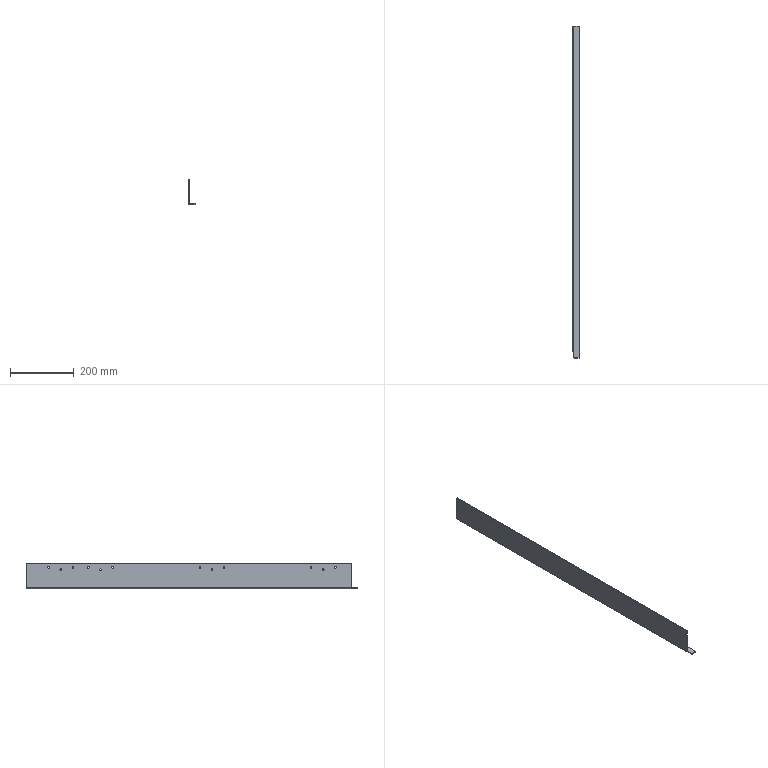Part | STEP file | HESS-408-70-15W-W-6-outer case reinforcing rib 2 | 1 solid | 37 faces | box 20 x 1043 x 80 mm | volume 295868 mm3 | cylinder 27 | plane 10 | commonest cylinder face diameters 5 x24 0.2 x1 2 x1 6.2 x1